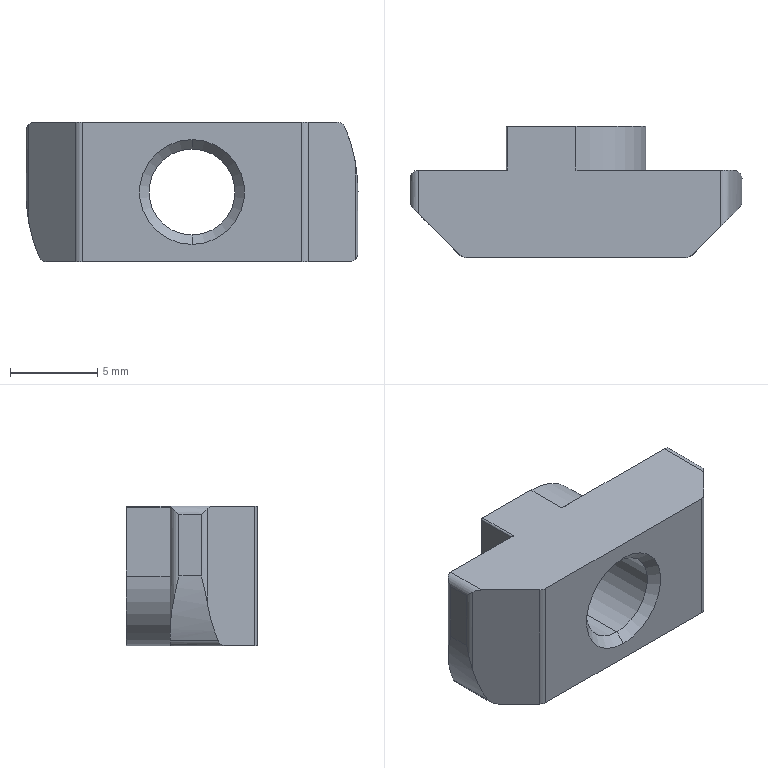Part | SolidWorks | features ICE 2, Extrusion 1, RevCut 1 | 1 solid | 34 faces | box 19 x 7.5 x 7.999 mm | volume 677.198 mm3 | cylinder 18 | plane 12 | cone 4 | commonest cylinder face diameters 1 x10 0.2 x2 4.917 x2 8 x2 19 x2
STEP:
#1=CARTESIAN_POINT('',(0.,0.5415,-2.458));
#2=VERTEX_POINT('',#1);
#3=CARTESIAN_POINT('',(0.,0.5415,2.458));
#4=VERTEX_POINT('',#3);
#5=CARTESIAN_POINT('',(0.,0.5415,0.));
#6=DIRECTION('',(0.,1.,0.));
#7=DIRECTION('',(0.,0.,1.));
#8=AXIS2_PLACEMENT_3D('',#5,#6,#7);
#9=CIRCLE('',#8,2.458);
#10=EDGE_CURVE('',#2,#4,#9,.T.);
#11=ORIENTED_EDGE('',*,*,#10,.T.);
#12=CARTESIAN_POINT('',(0.,0.,3.));
#13=VERTEX_POINT('',#12);
#14=CARTESIAN_POINT('',(0.,0.,3.));
#15=DIRECTION('',(0.,-0.7071,0.7071));
#16=VECTOR('',#15,1000.);
#17=LINE('',#14,#16);
#18=EDGE_CURVE('',#4,#13,#17,.T.);
#19=ORIENTED_EDGE('',*,*,#18,.T.);
#20=CARTESIAN_POINT('',(0.,0.,-3.));
#21=VERTEX_POINT('',#20);
#22=CARTESIAN_POINT('',(0.,0.,0.));
#23=DIRECTION('',(0.,1.,0.));
#24=DIRECTION('',(0.,0.,1.));
#25=AXIS2_PLACEMENT_3D('',#22,#23,#24);
#26=CIRCLE('',#25,3.);
#27=EDGE_CURVE('',#21,#13,#26,.T.);
#28=ORIENTED_EDGE('',*,*,#27,.F.);
#29=CARTESIAN_POINT('',(0.,0.,-3.));
#30=DIRECTION('',(0.,-0.7071,-0.7071));
#31=VECTOR('',#30,1000.);
#32=LINE('',#29,#31);
#33=EDGE_CURVE('',#2,#21,#32,.T.);
#34=ORIENTED_EDGE('',*,*,#33,.F.);
#35=EDGE_LOOP('',(#11,#19,#28,#34));
#36=FACE_OUTER_BOUND('',#35,.T.);
#37=CARTESIAN_POINT('',(0.,0.,0.));
#38=DIRECTION('',(0.,-1.,0.));
#39=DIRECTION('',(0.,0.,-1.));
#40=AXIS2_PLACEMENT_3D('',#37,#38,#39);
#41=CONICAL_SURFACE('',#40,3.,0.7854);
#42=ADVANCED_FACE('',(#36),#41,.F.);
#43=ORIENTED_EDGE('',*,*,#10,.F.);
#44=CARTESIAN_POINT('',(0.,6.958,-2.458));
#45=VERTEX_POINT('',#44);
#46=CARTESIAN_POINT('',(0.,0.,-2.458));
#47=DIRECTION('',(0.,1.,0.));
#48=VECTOR('',#47,1000.);
#49=LINE('',#46,#48);
#50=EDGE_CURVE('',#2,#45,#49,.T.);
#51=ORIENTED_EDGE('',*,*,#50,.T.);
#52=CARTESIAN_POINT('',(0.,6.958,2.458));
#53=VERTEX_POINT('',#52);
#54=CARTESIAN_POINT('',(0.,6.958,0.));
#55=DIRECTION('',(0.,1.,0.));
#56=DIRECTION('',(0.,0.,1.));
#57=AXIS2_PLACEMENT_3D('',#54,#55,#56);
#58=CIRCLE('',#57,2.458);
#59=EDGE_CURVE('',#45,#53,#58,.T.);
#60=ORIENTED_EDGE('',*,*,#59,.T.);
#61=CARTESIAN_POINT('',(0.,0.,2.458));
#62=DIRECTION('',(0.,1.,0.));
#63=VECTOR('',#62,1000.);
#64=LINE('',#61,#63);
#65=EDGE_CURVE('',#4,#53,#64,.T.);
#66=ORIENTED_EDGE('',*,*,#65,.F.);
#67=EDGE_LOOP('',(#43,#51,#60,#66));
#68=FACE_OUTER_BOUND('',#67,.T.);
#69=CARTESIAN_POINT('',(0.,0.,0.));
#70=DIRECTION('',(0.,1.,0.));
#71=DIRECTION('',(0.,0.,1.));
#72=AXIS2_PLACEMENT_3D('',#69,#70,#71);
#73=CYLINDRICAL_SURFACE('',#72,2.458);
#74=ADVANCED_FACE('',(#68),#73,.F.);
#75=ORIENTED_EDGE('',*,*,#59,.F.);
#76=CARTESIAN_POINT('',(0.,7.5,-3.));
#77=VERTEX_POINT('',#76);
#78=CARTESIAN_POINT('',(0.,6.958,-2.458));
#79=DIRECTION('',(0.,0.7071,-0.7071));
#80=VECTOR('',#79,1000.);
#81=LINE('',#78,#80);
#82=EDGE_CURVE('',#45,#77,#81,.T.);
#83=ORIENTED_EDGE('',*,*,#82,.T.);
#84=CARTESIAN_POINT('',(0.,7.5,3.));
#85=VERTEX_POINT('',#84);
#86=CARTESIAN_POINT('',(0.,7.5,0.));
#87=DIRECTION('',(0.,1.,0.));
#88=DIRECTION('',(0.,0.,1.));
#89=AXIS2_PLACEMENT_3D('',#86,#87,#88);
#90=CIRCLE('',#89,3.);
#91=EDGE_CURVE('',#77,#85,#90,.T.);
#92=ORIENTED_EDGE('',*,*,#91,.T.);
#93=CARTESIAN_POINT('',(0.,6.958,2.458));
#94=DIRECTION('',(0.,0.7071,0.7071));
#95=VECTOR('',#94,1000.);
#96=LINE('',#93,#95);
#97=EDGE_CURVE('',#53,#85,#96,.T.);
#98=ORIENTED_EDGE('',*,*,#97,.F.);
#99=EDGE_LOOP('',(#75,#83,#92,#98));
#100=FACE_OUTER_BOUND('',#99,.T.);
#101=CARTESIAN_POINT('',(0.,6.958,0.));
#102=DIRECTION('',(0.,1.,0.));
#103=DIRECTION('',(0.,0.,1.));
#104=AXIS2_PLACEMENT_3D('',#101,#102,#103);
#105=CONICAL_SURFACE('',#104,2.458,0.7854);
#106=ADVANCED_FACE('',(#100),#105,.F.);
#107=CARTESIAN_POINT('',(-6.646,0.1464,3.999));
#108=VERTEX_POINT('',#107);
#109=CARTESIAN_POINT('',(-9.,2.5,3.999));
#110=VERTEX_POINT('',#109);
#111=CARTESIAN_POINT('',(-9.354,2.854,3.999));
#112=DIRECTION('',(-0.7071,0.7071,0.));
#113=VECTOR('',#112,1000.);
#114=LINE('',#111,#113);
#115=EDGE_CURVE('',#108,#110,#114,.T.);
#116=ORIENTED_EDGE('',*,*,#115,.T.);
#117=CARTESIAN_POINT('',(-9.354,2.854,3.852));
#118=VERTEX_POINT('',#117);
#119=CARTESIAN_POINT('',(-9.,2.5,3.999));
#120=CARTESIAN_POINT('',(-9.134,2.634,3.999));
#121=CARTESIAN_POINT('',(-9.259,2.759,3.947));
#122=CARTESIAN_POINT('',(-9.354,2.854,3.852));
#123=(BOUNDED_CURVE()B_SPLINE_CURVE(3,(#119,#120,#121,#122),.UNSPECIFIED.,.F.,.F.)B_SPLINE_CURVE_WITH_KNOTS((4,4),(1.571,2.356),.UNSPECIFIED.)CURVE()GEOMETRIC_REPRESENTATION_ITEM()RATIONAL_B_SPLINE_CURVE((1.,0.9493,0.9493,1.))REPRESENTATION_ITEM(''));
#124=EDGE_CURVE('',#110,#118,#123,.T.);
#125=ORIENTED_EDGE('',*,*,#124,.T.);
#126=CARTESIAN_POINT('',(-9.354,2.854,-1.662));
#127=VERTEX_POINT('',#126);
#128=CARTESIAN_POINT('',(-9.354,2.854,4.));
#129=DIRECTION('',(0.,0.,-1.));
#130=VECTOR('',#129,1000.);
#131=LINE('',#128,#130);
#132=EDGE_CURVE('',#118,#127,#131,.T.);
#133=ORIENTED_EDGE('',*,*,#132,.T.);
#134=CARTESIAN_POINT('',(-8.752,2.252,-3.695));
#135=VERTEX_POINT('',#134);
#136=CARTESIAN_POINT('',(-9.354,2.854,-1.662));
#137=CARTESIAN_POINT('',(-9.229,2.729,-2.361));
#138=CARTESIAN_POINT('',(-9.028,2.528,-3.042));
#139=CARTESIAN_POINT('',(-8.752,2.252,-3.695));
#140=(BOUNDED_CURVE()B_SPLINE_CURVE(3,(#136,#137,#138,#139),.UNSPECIFIED.,.F.,.T.)B_SPLINE_CURVE_WITH_KNOTS((4,4),(3.317,3.541),.UNSPECIFIED.)CURVE()GEOMETRIC_REPRESENTATION_ITEM()RATIONAL_B_SPLINE_CURVE((1.,0.9958,0.9958,1.))REPRESENTATION_ITEM(''));
#141=EDGE_CURVE('',#127,#135,#140,.T.);
#142=ORIENTED_EDGE('',*,*,#141,.T.);
#143=CARTESIAN_POINT('',(-8.329,1.829,-4.));
#144=VERTEX_POINT('',#143);
#145=CARTESIAN_POINT('',(-8.752,2.252,-3.695));
#146=CARTESIAN_POINT('',(-8.677,2.177,-3.873));
#147=CARTESIAN_POINT('',(-8.521,2.021,-3.985));
#148=CARTESIAN_POINT('',(-8.329,1.829,-4.));
#149=(BOUNDED_CURVE()B_SPLINE_CURVE(3,(#145,#146,#147,#148),.UNSPECIFIED.,.F.,.F.)B_SPLINE_CURVE_WITH_KNOTS((4,4),(3.54,4.636),.UNSPECIFIED.)CURVE()GEOMETRIC_REPRESENTATION_ITEM()RATIONAL_B_SPLINE_CURVE((1.,0.9023,0.9023,1.))REPRESENTATION_ITEM(''));
#150=EDGE_CURVE('',#135,#144,#149,.T.);
#151=ORIENTED_EDGE('',*,*,#150,.T.);
#152=CARTESIAN_POINT('',(-6.646,0.1464,-4.));
#153=VERTEX_POINT('',#152);
#154=CARTESIAN_POINT('',(-9.354,2.854,-4.));
#155=DIRECTION('',(0.7071,-0.7071,0.));
#156=VECTOR('',#155,1000.);
#157=LINE('',#154,#156);
#158=EDGE_CURVE('',#144,#153,#157,.T.);
#159=ORIENTED_EDGE('',*,*,#158,.T.);
#160=CARTESIAN_POINT('',(-6.646,0.1464,4.));
#161=DIRECTION('',(0.,0.,-1.));
#162=VECTOR('',#161,1000.);
#163=LINE('',#160,#162);
#164=EDGE_CURVE('',#108,#153,#163,.T.);
#165=ORIENTED_EDGE('',*,*,#164,.F.);
#166=EDGE_LOOP('',(#116,#125,#133,#142,#151,#159,#165));
#167=FACE_OUTER_BOUND('',#166,.T.);
#168=CARTESIAN_POINT('',(-9.354,2.854,4.));
#169=DIRECTION('',(0.7071,0.7071,0.));
#170=DIRECTION('',(-0.7071,0.7071,0.));
#171=AXIS2_PLACEMENT_3D('',#168,#169,#170);
#172=PLANE('',#171);
#173=ADVANCED_FACE('',(#167),#172,.F.);
#174=CARTESIAN_POINT('',(8.753,2.252,3.693));
#175=VERTEX_POINT('',#174);
#176=CARTESIAN_POINT('',(8.292,1.791,3.999));
#177=VERTEX_POINT('',#176);
#178=CARTESIAN_POINT('',(8.753,2.252,3.693));
#179=CARTESIAN_POINT('',(8.672,2.171,3.884));
#180=CARTESIAN_POINT('',(8.5,1.999,3.999));
#181=CARTESIAN_POINT('',(8.292,1.791,3.999));
#182=(BOUNDED_CURVE()B_SPLINE_CURVE(3,(#178,#179,#180,#181),.UNSPECIFIED.,.F.,.F.)B_SPLINE_CURVE_WITH_KNOTS((4,4),(3.54,4.712),.UNSPECIFIED.)CURVE()GEOMETRIC_REPRESENTATION_ITEM()RATIONAL_B_SPLINE_CURVE((1.,0.8887,0.8887,1.))REPRESENTATION_ITEM(''));
#183=EDGE_CURVE('',#175,#177,#182,.T.);
#184=ORIENTED_EDGE('',*,*,#183,.T.);
#185=CARTESIAN_POINT('',(6.647,0.1464,3.999));
#186=VERTEX_POINT('',#185);
#187=CARTESIAN_POINT('',(6.647,0.1464,3.999));
#188=DIRECTION('',(-0.7071,-0.7071,0.));
#189=VECTOR('',#188,1000.);
#190=LINE('',#187,#189);
#191=EDGE_CURVE('',#177,#186,#190,.T.);
#192=ORIENTED_EDGE('',*,*,#191,.T.);
#193=CARTESIAN_POINT('',(6.647,0.1464,-4.));
#194=VERTEX_POINT('',#193);
#195=CARTESIAN_POINT('',(6.647,0.1464,4.));
#196=DIRECTION('',(0.,0.,-1.));
#197=VECTOR('',#196,1000.);
#198=LINE('',#195,#197);
#199=EDGE_CURVE('',#186,#194,#198,.T.);
#200=ORIENTED_EDGE('',*,*,#199,.T.);
#201=CARTESIAN_POINT('',(9.038,2.537,-4.));
#202=VERTEX_POINT('',#201);
#203=CARTESIAN_POINT('',(6.647,0.1464,-4.));
#204=DIRECTION('',(0.7071,0.7071,0.));
#205=VECTOR('',#204,1000.);
#206=LINE('',#203,#205);
#207=EDGE_CURVE('',#194,#202,#206,.T.);
#208=ORIENTED_EDGE('',*,*,#207,.T.);
#209=CARTESIAN_POINT('',(9.354,2.853,-3.855));
#210=VERTEX_POINT('',#209);
#211=CARTESIAN_POINT('',(9.038,2.537,-4.));
#212=CARTESIAN_POINT('',(9.158,2.657,-3.991));
#213=CARTESIAN_POINT('',(9.268,2.767,-3.94));
#214=CARTESIAN_POINT('',(9.354,2.853,-3.855));
#215=(BOUNDED_CURVE()B_SPLINE_CURVE(3,(#211,#212,#213,#214),.UNSPECIFIED.,.F.,.F.)B_SPLINE_CURVE_WITH_KNOTS((4,4),(1.647,2.356),.UNSPECIFIED.)CURVE()GEOMETRIC_REPRESENTATION_ITEM()RATIONAL_B_SPLINE_CURVE((1.,0.9585,0.9585,1.))REPRESENTATION_ITEM(''));
#216=EDGE_CURVE('',#202,#210,#215,.T.);
#217=ORIENTED_EDGE('',*,*,#216,.T.);
#218=CARTESIAN_POINT('',(9.354,2.853,1.662));
#219=VERTEX_POINT('',#218);
#220=CARTESIAN_POINT('',(9.354,2.853,4.));
#221=DIRECTION('',(0.,0.,-1.));
#222=VECTOR('',#221,1000.);
#223=LINE('',#220,#222);
#224=EDGE_CURVE('',#219,#210,#223,.T.);
#225=ORIENTED_EDGE('',*,*,#224,.F.);
#226=CARTESIAN_POINT('',(9.354,2.853,1.662));
#227=CARTESIAN_POINT('',(9.23,2.729,2.36));
#228=CARTESIAN_POINT('',(9.029,2.528,3.039));
#229=CARTESIAN_POINT('',(8.753,2.252,3.693));
#230=(BOUNDED_CURVE()B_SPLINE_CURVE(3,(#226,#227,#228,#229),.UNSPECIFIED.,.F.,.F.)B_SPLINE_CURVE_WITH_KNOTS((4,4),(3.317,3.541),.UNSPECIFIED.)CURVE()GEOMETRIC_REPRESENTATION_ITEM()RATIONAL_B_SPLINE_CURVE((1.,0.9958,0.9958,1.))REPRESENTATION_ITEM(''));
#231=EDGE_CURVE('',#219,#175,#230,.T.);
#232=ORIENTED_EDGE('',*,*,#231,.T.);
#233=EDGE_LOOP('',(#184,#192,#200,#208,#217,#225,#232));
#234=FACE_OUTER_BOUND('',#233,.T.);
#235=CARTESIAN_POINT('',(6.647,0.1464,4.));
#236=DIRECTION('',(-0.7071,0.7071,0.));
#237=DIRECTION('',(-0.7071,-0.7071,0.));
#238=AXIS2_PLACEMENT_3D('',#235,#236,#237);
#239=PLANE('',#238);
#240=ADVANCED_FACE('',(#234),#239,.F.);
#241=CARTESIAN_POINT('',(9.5,4.5,-3.501));
#242=VERTEX_POINT('',#241);
#243=CARTESIAN_POINT('',(9.5,3.206,-3.501));
#244=VERTEX_POINT('',#243);
#245=CARTESIAN_POINT('',(9.5,5.5,-3.501));
#246=DIRECTION('',(0.,-1.,0.));
#247=VECTOR('',#246,1000.);
#248=LINE('',#245,#247);
#249=EDGE_CURVE('',#242,#244,#248,.T.);
#250=ORIENTED_EDGE('',*,*,#249,.F.);
#251=CARTESIAN_POINT('',(9.5,4.5,0.));
#252=VERTEX_POINT('',#251);
#253=CARTESIAN_POINT('',(9.5,4.5,4.));
#254=DIRECTION('',(0.,0.,-1.));
#255=VECTOR('',#254,1000.);
#256=LINE('',#253,#255);
#257=EDGE_CURVE('',#252,#242,#256,.T.);
#258=ORIENTED_EDGE('',*,*,#257,.F.);
#259=CARTESIAN_POINT('',(9.5,3.206,0.));
#260=VERTEX_POINT('',#259);
#261=CARTESIAN_POINT('',(9.5,5.5,0.));
#262=DIRECTION('',(0.,1.,0.));
#263=VECTOR('',#262,1000.);
#264=LINE('',#261,#263);
#265=EDGE_CURVE('',#260,#252,#264,.T.);
#266=ORIENTED_EDGE('',*,*,#265,.F.);
#267=CARTESIAN_POINT('',(9.5,3.206,4.));
#268=DIRECTION('',(0.,0.,-1.));
#269=VECTOR('',#268,1000.);
#270=LINE('',#267,#269);
#271=EDGE_CURVE('',#260,#244,#270,.T.);
#272=ORIENTED_EDGE('',*,*,#271,.T.);
#273=EDGE_LOOP('',(#250,#258,#266,#272));
#274=FACE_OUTER_BOUND('',#273,.T.);
#275=CARTESIAN_POINT('',(9.5,3.206,4.));
#276=DIRECTION('',(-1.,0.,0.));
#277=DIRECTION('',(0.,0.,1.));
#278=AXIS2_PLACEMENT_3D('',#275,#276,#277);
#279=PLANE('',#278);
#280=ADVANCED_FACE('',(#274),#279,.F.);
#281=CARTESIAN_POINT('',(-9.,5.,3.999));
#282=VERTEX_POINT('',#281);
#283=CARTESIAN_POINT('',(-9.,5.,-3.042));
#284=VERTEX_POINT('',#283);
#285=CARTESIAN_POINT('',(-9.,5.,4.));
#286=DIRECTION('',(0.,0.,-1.));
#287=VECTOR('',#286,1000.);
#288=LINE('',#285,#287);
#289=EDGE_CURVE('',#282,#284,#288,.T.);
#290=ORIENTED_EDGE('',*,*,#289,.F.);
#291=CARTESIAN_POINT('',(-3.9,5.,3.999));
#292=VERTEX_POINT('',#291);
#293=CARTESIAN_POINT('',(-4.1,5.,3.999));
#294=DIRECTION('',(1.,0.,0.));
#295=VECTOR('',#294,1000.);
#296=LINE('',#293,#295);
#297=EDGE_CURVE('',#282,#292,#296,.T.);
#298=ORIENTED_EDGE('',*,*,#297,.T.);
#299=CARTESIAN_POINT('',(-4.,5.,3.899));
#300=VERTEX_POINT('',#299);
#301=CARTESIAN_POINT('',(-3.9,5.,3.899));
#302=DIRECTION('',(0.,1.,0.));
#303=DIRECTION('',(0.,0.,1.));
#304=AXIS2_PLACEMENT_3D('',#301,#302,#303);
#305=CIRCLE('',#304,0.1);
#306=EDGE_CURVE('',#300,#292,#305,.T.);
#307=ORIENTED_EDGE('',*,*,#306,.F.);
#308=CARTESIAN_POINT('',(-4.,5.,-0.001441));
#309=VERTEX_POINT('',#308);
#310=CARTESIAN_POINT('',(-4.,5.,-0.001441));
#311=DIRECTION('',(0.,0.,1.));
#312=VECTOR('',#311,1000.);
#313=LINE('',#310,#312);
#314=EDGE_CURVE('',#309,#300,#313,.T.);
#315=ORIENTED_EDGE('',*,*,#314,.F.);
#316=CARTESIAN_POINT('',(-0.1074,5.,-4.));
#317=VERTEX_POINT('',#316);
#318=CARTESIAN_POINT('',(-0.000000109,5.,-0.001441));
#319=DIRECTION('',(0.,1.,0.));
#320=DIRECTION('',(0.,0.,1.));
#321=AXIS2_PLACEMENT_3D('',#318,#319,#320);
#322=CIRCLE('',#321,4.);
#323=EDGE_CURVE('',#317,#309,#322,.T.);
#324=ORIENTED_EDGE('',*,*,#323,.F.);
#325=CARTESIAN_POINT('',(-8.329,5.,-4.));
#326=VERTEX_POINT('',#325);
#327=CARTESIAN_POINT('',(-4.1,5.,-4.));
#328=DIRECTION('',(-1.,0.,0.));
#329=VECTOR('',#328,1000.);
#330=LINE('',#327,#329);
#331=EDGE_CURVE('',#317,#326,#330,.T.);
#332=ORIENTED_EDGE('',*,*,#331,.T.);
#333=CARTESIAN_POINT('',(-8.752,5.,-3.695));
#334=VERTEX_POINT('',#333);
#335=CARTESIAN_POINT('',(-8.291,5.,-3.501));
#336=DIRECTION('',(0.,1.,0.));
#337=DIRECTION('',(0.,0.,-1.));
#338=AXIS2_PLACEMENT_3D('',#335,#336,#337);
#339=CIRCLE('',#338,0.5);
#340=EDGE_CURVE('',#326,#334,#339,.T.);
#341=ORIENTED_EDGE('',*,*,#340,.T.);
#342=CARTESIAN_POINT('',(-0.000000132,5.,-0.0005123));
#343=DIRECTION('',(0.,1.,0.));
#344=DIRECTION('',(0.,0.,-1.));
#345=AXIS2_PLACEMENT_3D('',#342,#343,#344);
#346=CIRCLE('',#345,9.5);
#347=EDGE_CURVE('',#334,#284,#346,.T.);
#348=ORIENTED_EDGE('',*,*,#347,.T.);
#349=EDGE_LOOP('',(#290,#298,#307,#315,#324,#332,#341,#348));
#350=FACE_OUTER_BOUND('',#349,.T.);
#351=CARTESIAN_POINT('',(-4.1,5.,4.));
#352=DIRECTION('',(0.,-1.,0.));
#353=DIRECTION('',(0.,0.,-1.));
#354=AXIS2_PLACEMENT_3D('',#351,#352,#353);
#355=PLANE('',#354);
#356=ADVANCED_FACE('',(#350),#355,.F.);
#357=CARTESIAN_POINT('',(-0.000000109,5.,3.999));
#358=VERTEX_POINT('',#357);
#359=CARTESIAN_POINT('',(4.,5.,-0.001441));
#360=VERTEX_POINT('',#359);
#361=CARTESIAN_POINT('',(-0.000000109,5.,-0.001441));
#362=DIRECTION('',(0.,1.,0.));
#363=DIRECTION('',(0.,0.,1.));
#364=AXIS2_PLACEMENT_3D('',#361,#362,#363);
#365=CIRCLE('',#364,4.);
#366=EDGE_CURVE('',#358,#360,#365,.T.);
#367=ORIENTED_EDGE('',*,*,#366,.F.);
#368=CARTESIAN_POINT('',(8.292,5.,3.999));
#369=VERTEX_POINT('',#368);
#370=CARTESIAN_POINT('',(-4.1,5.,3.999));
#371=DIRECTION('',(1.,0.,0.));
#372=VECTOR('',#371,1000.);
#373=LINE('',#370,#372);
#374=EDGE_CURVE('',#358,#369,#373,.T.);
#375=ORIENTED_EDGE('',*,*,#374,.T.);
#376=CARTESIAN_POINT('',(8.753,5.,3.693));
#377=VERTEX_POINT('',#376);
#378=CARTESIAN_POINT('',(8.292,5.,3.499));
#379=DIRECTION('',(0.,1.,0.));
#380=DIRECTION('',(0.,0.,-1.));
#381=AXIS2_PLACEMENT_3D('',#378,#379,#380);
#382=CIRCLE('',#381,0.5);
#383=EDGE_CURVE('',#369,#377,#382,.T.);
#384=ORIENTED_EDGE('',*,*,#383,.T.);
#385=CARTESIAN_POINT('',(9.,5.,3.041));
#386=VERTEX_POINT('',#385);
#387=CARTESIAN_POINT('',(0.,5.,0.));
#388=DIRECTION('',(0.,1.,0.));
#389=DIRECTION('',(0.,0.,-1.));
#390=AXIS2_PLACEMENT_3D('',#387,#388,#389);
#391=CIRCLE('',#390,9.5);
#392=EDGE_CURVE('',#377,#386,#391,.T.);
#393=ORIENTED_EDGE('',*,*,#392,.T.);
#394=CARTESIAN_POINT('',(9.,5.,-4.));
#395=VERTEX_POINT('',#394);
#396=CARTESIAN_POINT('',(9.,5.,4.));
#397=DIRECTION('',(0.,0.,-1.));
#398=VECTOR('',#397,1000.);
#399=LINE('',#396,#398);
#400=EDGE_CURVE('',#386,#395,#399,.T.);
#401=ORIENTED_EDGE('',*,*,#400,.T.);
#402=CARTESIAN_POINT('',(3.917,5.,-4.));
#403=VERTEX_POINT('',#402);
#404=CARTESIAN_POINT('',(9.,5.,-4.));
#405=DIRECTION('',(-1.,0.,0.));
#406=VECTOR('',#405,1000.);
#407=LINE('',#404,#406);
#408=EDGE_CURVE('',#395,#403,#407,.T.);
#409=ORIENTED_EDGE('',*,*,#408,.T.);
#410=CARTESIAN_POINT('',(4.,5.,-3.901));
#411=VERTEX_POINT('',#410);
#412=CARTESIAN_POINT('',(3.9,5.,-3.901));
#413=DIRECTION('',(0.,1.,0.));
#414=DIRECTION('',(0.,0.,1.));
#415=AXIS2_PLACEMENT_3D('',#412,#413,#414);
#416=CIRCLE('',#415,0.1);
#417=EDGE_CURVE('',#411,#403,#416,.T.);
#418=ORIENTED_EDGE('',*,*,#417,.F.);
#419=CARTESIAN_POINT('',(4.,5.,-0.001441));
#420=DIRECTION('',(0.,0.,-1.));
#421=VECTOR('',#420,1000.);
#422=LINE('',#419,#421);
#423=EDGE_CURVE('',#360,#411,#422,.T.);
#424=ORIENTED_EDGE('',*,*,#423,.F.);
#425=EDGE_LOOP('',(#367,#375,#384,#393,#401,#409,#418,#424));
#426=FACE_OUTER_BOUND('',#425,.T.);
#427=CARTESIAN_POINT('',(-4.1,5.,4.));
#428=DIRECTION('',(0.,-1.,0.));
#429=DIRECTION('',(0.,0.,-1.));
#430=AXIS2_PLACEMENT_3D('',#427,#428,#429);
#431=PLANE('',#430);
#432=ADVANCED_FACE('',(#426),#431,.F.);
#433=CARTESIAN_POINT('',(-9.5,3.207,3.499));
#434=VERTEX_POINT('',#433);
#435=CARTESIAN_POINT('',(-9.5,3.207,-0.0005123));
#436=VERTEX_POINT('',#435);
#437=CARTESIAN_POINT('',(-9.5,3.207,4.));
#438=DIRECTION('',(0.,0.,-1.));
#439=VECTOR('',#438,1000.);
#440=LINE('',#437,#439);
#441=EDGE_CURVE('',#434,#436,#440,.T.);
#442=ORIENTED_EDGE('',*,*,#441,.F.);
#443=CARTESIAN_POINT('',(-9.5,4.5,3.499));
#444=VERTEX_POINT('',#443);
#445=CARTESIAN_POINT('',(-9.5,5.5,3.499));
#446=DIRECTION('',(0.,1.,0.));
#447=VECTOR('',#446,1000.);
#448=LINE('',#445,#447);
#449=EDGE_CURVE('',#434,#444,#448,.T.);
#450=ORIENTED_EDGE('',*,*,#449,.T.);
#451=CARTESIAN_POINT('',(-9.5,4.5,-0.0005123));
#452=VERTEX_POINT('',#451);
#453=CARTESIAN_POINT('',(-9.5,4.5,4.));
#454=DIRECTION('',(0.,0.,-1.));
#455=VECTOR('',#454,1000.);
#456=LINE('',#453,#455);
#457=EDGE_CURVE('',#444,#452,#456,.T.);
#458=ORIENTED_EDGE('',*,*,#457,.T.);
#459=CARTESIAN_POINT('',(-9.5,5.5,-0.0005123));
#460=DIRECTION('',(0.,1.,0.));
#461=VECTOR('',#460,1000.);
#462=LINE('',#459,#461);
#463=EDGE_CURVE('',#436,#452,#462,.T.);
#464=ORIENTED_EDGE('',*,*,#463,.F.);
#465=EDGE_LOOP('',(#442,#450,#458,#464));
#466=FACE_OUTER_BOUND('',#465,.T.);
#467=CARTESIAN_POINT('',(-9.5,4.5,4.));
#468=DIRECTION('',(1.,0.,0.));
#469=DIRECTION('',(0.,0.,-1.));
#470=AXIS2_PLACEMENT_3D('',#467,#468,#469);
#471=PLANE('',#470);
#472=ADVANCED_FACE('',(#466),#471,.F.);
#473=CARTESIAN_POINT('',(4.,7.5,-0.001441));
#474=VERTEX_POINT('',#473);
#475=CARTESIAN_POINT('',(4.,11.,-0.001441));
#476=DIRECTION('',(0.,-1.,0.));
#477=VECTOR('',#476,1000.);
#478=LINE('',#475,#477);
#479=EDGE_CURVE('',#474,#360,#478,.T.);
#480=ORIENTED_EDGE('',*,*,#479,.T.);
#481=ORIENTED_EDGE('',*,*,#423,.T.);
#482=CARTESIAN_POINT('',(4.,7.5,-3.901));
#483=VERTEX_POINT('',#482);
#484=CARTESIAN_POINT('',(4.,11.,-3.901));
#485=DIRECTION('',(0.,-1.,0.));
#486=VECTOR('',#485,1000.);
#487=LINE('',#484,#486);
#488=EDGE_CURVE('',#483,#411,#487,.T.);
#489=ORIENTED_EDGE('',*,*,#488,.F.);
#490=CARTESIAN_POINT('',(4.,7.5,4.));
#491=DIRECTION('',(0.,0.,-1.));
#492=VECTOR('',#491,1000.);
#493=LINE('',#490,#492);
#494=EDGE_CURVE('',#474,#483,#493,.T.);
#495=ORIENTED_EDGE('',*,*,#494,.F.);
#496=EDGE_LOOP('',(#480,#481,#489,#495));
#497=FACE_OUTER_BOUND('',#496,.T.);
#498=CARTESIAN_POINT('',(4.,5.1,4.));
#499=DIRECTION('',(-1.,0.,0.));
#500=DIRECTION('',(0.,0.,1.));
#501=AXIS2_PLACEMENT_3D('',#498,#499,#500);
#502=PLANE('',#501);
#503=ADVANCED_FACE('',(#497),#502,.F.);
#504=CARTESIAN_POINT('',(0.,7.5,0.));
#505=DIRECTION('',(0.,1.,0.));
#506=DIRECTION('',(0.,0.,1.));
#507=AXIS2_PLACEMENT_3D('',#504,#505,#506);
#508=CIRCLE('',#507,3.);
#509=EDGE_CURVE('',#85,#77,#508,.T.);
#510=ORIENTED_EDGE('',*,*,#509,.F.);
#511=ORIENTED_EDGE('',*,*,#91,.F.);
#512=EDGE_LOOP('',(#510,#511));
#513=FACE_BOUND('',#512,.T.);
#514=CARTESIAN_POINT('',(3.917,7.5,-4.));
#515=VERTEX_POINT('',#514);
#516=CARTESIAN_POINT('',(-0.1074,7.5,-4.));
#517=VERTEX_POINT('',#516);
#518=CARTESIAN_POINT('',(4.,7.5,-4.));
#519=DIRECTION('',(-1.,0.,0.));
#520=VECTOR('',#519,1000.);
#521=LINE('',#518,#520);
#522=EDGE_CURVE('',#515,#517,#521,.T.);
#523=ORIENTED_EDGE('',*,*,#522,.T.);
#524=CARTESIAN_POINT('',(-4.,7.5,-0.001441));
#525=VERTEX_POINT('',#524);
#526=CARTESIAN_POINT('',(-0.000000109,7.5,-0.001441));
#527=DIRECTION('',(0.,1.,0.));
#528=DIRECTION('',(0.,0.,-1.));
#529=AXIS2_PLACEMENT_3D('',#526,#527,#528);
#530=CIRCLE('',#529,4.);
#531=EDGE_CURVE('',#517,#525,#530,.T.);
#532=ORIENTED_EDGE('',*,*,#531,.T.);
#533=CARTESIAN_POINT('',(-4.,7.5,3.899));
#534=VERTEX_POINT('',#533);
#535=CARTESIAN_POINT('',(-4.,7.5,4.));
#536=DIRECTION('',(0.,0.,-1.));
#537=VECTOR('',#536,1000.);
#538=LINE('',#535,#537);
#539=EDGE_CURVE('',#534,#525,#538,.T.);
#540=ORIENTED_EDGE('',*,*,#539,.F.);
#541=CARTESIAN_POINT('',(-3.9,7.5,3.999));
#542=VERTEX_POINT('',#541);
#543=CARTESIAN_POINT('',(-3.9,7.5,3.899));
#544=DIRECTION('',(0.,1.,0.));
#545=DIRECTION('',(0.,0.,-1.));
#546=AXIS2_PLACEMENT_3D('',#543,#544,#545);
#547=CIRCLE('',#546,0.1);
#548=EDGE_CURVE('',#534,#542,#547,.T.);
#549=ORIENTED_EDGE('',*,*,#548,.T.);
#550=CARTESIAN_POINT('',(-0.000000109,7.5,3.999));
#551=VERTEX_POINT('',#550);
#552=CARTESIAN_POINT('',(4.,7.5,3.999));
#553=DIRECTION('',(1.,0.,0.));
#554=VECTOR('',#553,1000.);
#555=LINE('',#552,#554);
#556=EDGE_CURVE('',#542,#551,#555,.T.);
#557=ORIENTED_EDGE('',*,*,#556,.T.);
#558=CARTESIAN_POINT('',(-0.000000109,7.5,-0.001441));
#559=DIRECTION('',(0.,1.,0.));
#560=DIRECTION('',(0.,0.,-1.));
#561=AXIS2_PLACEMENT_3D('',#558,#559,#560);
#562=CIRCLE('',#561,4.);
#563=EDGE_CURVE('',#551,#474,#562,.T.);
#564=ORIENTED_EDGE('',*,*,#563,.T.);
#565=ORIENTED_EDGE('',*,*,#494,.T.);
#566=CARTESIAN_POINT('',(3.9,7.5,-3.901));
#567=DIRECTION('',(0.,1.,0.));
#568=DIRECTION('',(0.,0.,-1.));
#569=AXIS2_PLACEMENT_3D('',#566,#567,#568);
#570=CIRCLE('',#569,0.1);
#571=EDGE_CURVE('',#483,#515,#570,.T.);
#572=ORIENTED_EDGE('',*,*,#571,.T.);
#573=EDGE_LOOP('',(#523,#532,#540,#549,#557,#564,#565,#572));
#574=FACE_OUTER_BOUND('',#573,.T.);
#575=CARTESIAN_POINT('',(4.,7.5,4.));
#576=DIRECTION('',(0.,-1.,0.));
#577=DIRECTION('',(0.,0.,-1.));
#578=AXIS2_PLACEMENT_3D('',#575,#576,#577);
#579=PLANE('',#578);
#580=ADVANCED_FACE('',(#513,#574),#579,.F.);
#581=CARTESIAN_POINT('',(-4.,11.,-0.001441));
#582=DIRECTION('',(0.,-1.,0.));
#583=VECTOR('',#582,1000.);
#584=LINE('',#581,#583);
#585=EDGE_CURVE('',#525,#309,#584,.T.);
#586=ORIENTED_EDGE('',*,*,#585,.T.);
#587=ORIENTED_EDGE('',*,*,#314,.T.);
#588=CARTESIAN_POINT('',(-4.,11.,3.899));
#589=DIRECTION('',(0.,-1.,0.));
#590=VECTOR('',#589,1000.);
#591=LINE('',#588,#590);
#592=EDGE_CURVE('',#534,#300,#591,.T.);
#593=ORIENTED_EDGE('',*,*,#592,.F.);
#594=ORIENTED_EDGE('',*,*,#539,.T.);
#595=EDGE_LOOP('',(#586,#587,#593,#594));
#596=FACE_OUTER_BOUND('',#595,.T.);
#597=CARTESIAN_POINT('',(-4.,7.5,4.));
#598=DIRECTION('',(1.,0.,0.));
#599=DIRECTION('',(0.,0.,-1.));
#600=AXIS2_PLACEMENT_3D('',#597,#598,#599);
#601=PLANE('',#600);
#602=ADVANCED_FACE('',(#596),#601,.F.);
#603=CARTESIAN_POINT('',(9.038,4.999,-4.));
#604=VERTEX_POINT('',#603);
#605=CARTESIAN_POINT('',(9.,4.5,-4.));
#606=DIRECTION('',(0.,0.,1.));
#607=DIRECTION('',(1.,0.,0.));
#608=AXIS2_PLACEMENT_3D('',#605,#606,#607);
#609=CIRCLE('',#608,0.5);
#610=EDGE_CURVE('',#604,#395,#609,.T.);
#611=ORIENTED_EDGE('',*,*,#610,.F.);
#612=CARTESIAN_POINT('',(9.038,5.5,-4.));
#613=DIRECTION('',(0.,-1.,0.));
#614=VECTOR('',#613,1000.);
#615=LINE('',#612,#614);
#616=EDGE_CURVE('',#604,#202,#615,.T.);
#617=ORIENTED_EDGE('',*,*,#616,.T.);
#618=ORIENTED_EDGE('',*,*,#207,.F.);
#619=CARTESIAN_POINT('',(6.294,0.,-4.));
#620=VERTEX_POINT('',#619);
#621=CARTESIAN_POINT('',(6.294,0.5,-4.));
#622=DIRECTION('',(0.,0.,1.));
#623=DIRECTION('',(1.,0.,0.));
#624=AXIS2_PLACEMENT_3D('',#621,#622,#623);
#625=CIRCLE('',#624,0.5);
#626=EDGE_CURVE('',#620,#194,#625,.T.);
#627=ORIENTED_EDGE('',*,*,#626,.F.);
#628=CARTESIAN_POINT('',(-6.293,0.,-4.));
#629=VERTEX_POINT('',#628);
#630=CARTESIAN_POINT('',(-6.293,0.,-4.));
#631=DIRECTION('',(1.,0.,0.));
#632=VECTOR('',#631,1000.);
#633=LINE('',#630,#632);
#634=EDGE_CURVE('',#629,#620,#633,.T.);
#635=ORIENTED_EDGE('',*,*,#634,.F.);
#636=CARTESIAN_POINT('',(-6.293,0.5,-4.));
#637=DIRECTION('',(0.,0.,1.));
#638=DIRECTION('',(1.,0.,0.));
#639=AXIS2_PLACEMENT_3D('',#636,#637,#638);
#640=CIRCLE('',#639,0.5);
#641=EDGE_CURVE('',#153,#629,#640,.T.);
#642=ORIENTED_EDGE('',*,*,#641,.F.);
#643=ORIENTED_EDGE('',*,*,#158,.F.);
#644=CARTESIAN_POINT('',(-8.329,5.5,-4.));
#645=DIRECTION('',(0.,1.,0.));
#646=VECTOR('',#645,1000.);
#647=LINE('',#644,#646);
#648=EDGE_CURVE('',#144,#326,#647,.T.);
#649=ORIENTED_EDGE('',*,*,#648,.T.);
#650=ORIENTED_EDGE('',*,*,#331,.F.);
#651=CARTESIAN_POINT('',(-0.1074,11.,-4.));
#652=DIRECTION('',(0.,1.,0.));
#653=VECTOR('',#652,1000.);
#654=LINE('',#651,#653);
#655=EDGE_CURVE('',#317,#517,#654,.T.);
#656=ORIENTED_EDGE('',*,*,#655,.T.);
#657=ORIENTED_EDGE('',*,*,#522,.F.);
#658=CARTESIAN_POINT('',(3.917,11.,-4.));
#659=DIRECTION('',(0.,-1.,0.));
#660=VECTOR('',#659,1000.);
#661=LINE('',#658,#660);
#662=EDGE_CURVE('',#515,#403,#661,.T.);
#663=ORIENTED_EDGE('',*,*,#662,.T.);
#664=ORIENTED_EDGE('',*,*,#408,.F.);
#665=EDGE_LOOP('',(#611,#617,#618,#627,#635,#642,#643,#649,#650,#656,#657,#663,#664));
#666=FACE_OUTER_BOUND('',#665,.T.);
#667=CARTESIAN_POINT('',(-9.,3.207,-4.));
#668=DIRECTION('',(0.,0.,1.));
#669=DIRECTION('',(1.,0.,0.));
#670=AXIS2_PLACEMENT_3D('',#667,#668,#669);
#671=PLANE('',#670);
#672=ADVANCED_FACE('',(#666),#671,.F.);
#673=ORIENTED_EDGE('',*,*,#132,.F.);
#674=CARTESIAN_POINT('',(-9.354,2.854,3.852));
#675=CARTESIAN_POINT('',(-9.449,2.949,3.757));
#676=CARTESIAN_POINT('',(-9.5,3.073,3.633));
#677=CARTESIAN_POINT('',(-9.5,3.207,3.499));
#678=(BOUNDED_CURVE()B_SPLINE_CURVE(3,(#674,#675,#676,#677),.UNSPECIFIED.,.F.,.F.)B_SPLINE_CURVE_WITH_KNOTS((4,4),(3.927,4.712),.UNSPECIFIED.)CURVE()GEOMETRIC_REPRESENTATION_ITEM()RATIONAL_B_SPLINE_CURVE((1.,0.9493,0.9493,1.))REPRESENTATION_ITEM(''));
#679=EDGE_CURVE('',#118,#434,#678,.T.);
#680=ORIENTED_EDGE('',*,*,#679,.T.);
#681=ORIENTED_EDGE('',*,*,#441,.T.);
#682=CARTESIAN_POINT('',(-9.5,3.207,-0.0005123));
#683=CARTESIAN_POINT('',(-9.5,3.08,-0.5554));
#684=CARTESIAN_POINT('',(-9.452,2.952,-1.11));
#685=CARTESIAN_POINT('',(-9.354,2.854,-1.662));
#686=B_SPLINE_CURVE_WITH_KNOTS('',3,(#682,#683,#684,#685),.UNSPECIFIED.,.F.,.F.,(4,4),(-0.00001949,0.001688),.UNSPECIFIED.);
#687=EDGE_CURVE('',#436,#127,#686,.T.);
#688=ORIENTED_EDGE('',*,*,#687,.T.);
#689=EDGE_LOOP('',(#673,#680,#681,#688));
#690=FACE_OUTER_BOUND('',#689,.T.);
#691=CARTESIAN_POINT('',(-9.,3.207,4.));
#692=DIRECTION('',(0.,0.,-1.));
#693=DIRECTION('',(-1.,0.,0.));
#694=AXIS2_PLACEMENT_3D('',#691,#692,#693);
#695=CYLINDRICAL_SURFACE('',#694,0.5);
#696=ADVANCED_FACE('',(#690),#695,.T.);
#697=CARTESIAN_POINT('',(-6.293,0.,3.999));
#698=VERTEX_POINT('',#697);
#699=CARTESIAN_POINT('',(-6.293,0.,4.));
#700=DIRECTION('',(0.,0.,-1.));
#701=VECTOR('',#700,1000.);
#702=LINE('',#699,#701);
#703=EDGE_CURVE('',#698,#629,#702,.T.);
#704=ORIENTED_EDGE('',*,*,#703,.F.);
#705=CARTESIAN_POINT('',(-6.293,0.5,3.999));
#706=DIRECTION('',(0.,0.,-1.));
#707=DIRECTION('',(-1.,0.,0.));
#708=AXIS2_PLACEMENT_3D('',#705,#706,#707);
#709=CIRCLE('',#708,0.5);
#710=EDGE_CURVE('',#698,#108,#709,.T.);
#711=ORIENTED_EDGE('',*,*,#710,.T.);
#712=ORIENTED_EDGE('',*,*,#164,.T.);
#713=ORIENTED_EDGE('',*,*,#641,.T.);
#714=EDGE_LOOP('',(#704,#711,#712,#713));
#715=FACE_OUTER_BOUND('',#714,.T.);
#716=CARTESIAN_POINT('',(-6.293,0.5,4.));
#717=DIRECTION('',(0.,0.,-1.));
#718=DIRECTION('',(-1.,0.,0.));
#719=AXIS2_PLACEMENT_3D('',#716,#717,#718);
#720=CYLINDRICAL_SURFACE('',#719,0.5);
#721=ADVANCED_FACE('',(#715),#720,.T.);
#722=ORIENTED_EDGE('',*,*,#27,.T.);
#723=CARTESIAN_POINT('',(0.,0.,0.));
#724=DIRECTION('',(0.,1.,0.));
#725=DIRECTION('',(0.,0.,1.));
#726=AXIS2_PLACEMENT_3D('',#723,#724,#725);
#727=CIRCLE('',#726,3.);
#728=EDGE_CURVE('',#13,#21,#727,.T.);
#729=ORIENTED_EDGE('',*,*,#728,.T.);
#730=EDGE_LOOP('',(#722,#729));
#731=FACE_BOUND('',#730,.T.);
#732=CARTESIAN_POINT('',(6.294,0.,3.999));
#733=VERTEX_POINT('',#732);
#734=CARTESIAN_POINT('',(6.294,0.,4.));
#735=DIRECTION('',(0.,0.,-1.));
#736=VECTOR('',#735,1000.);
#737=LINE('',#734,#736);
#738=EDGE_CURVE('',#733,#620,#737,.T.);
#739=ORIENTED_EDGE('',*,*,#738,.F.);
#740=CARTESIAN_POINT('',(-9.,0.,3.999));
#741=DIRECTION('',(1.,0.,0.));
#742=VECTOR('',#741,1000.);
#743=LINE('',#740,#742);
#744=EDGE_CURVE('',#698,#733,#743,.T.);
#745=ORIENTED_EDGE('',*,*,#744,.F.);
#746=ORIENTED_EDGE('',*,*,#703,.T.);
#747=ORIENTED_EDGE('',*,*,#634,.T.);
#748=EDGE_LOOP('',(#739,#745,#746,#747));
#749=FACE_OUTER_BOUND('',#748,.T.);
#750=CARTESIAN_POINT('',(-6.293,0.,4.));
#751=DIRECTION('',(0.,1.,0.));
#752=DIRECTION('',(0.,0.,1.));
#753=AXIS2_PLACEMENT_3D('',#750,#751,#752);
#754=PLANE('',#753);
#755=ADVANCED_FACE('',(#731,#749),#754,.F.);
#756=ORIENTED_EDGE('',*,*,#199,.F.);
#757=CARTESIAN_POINT('',(6.294,0.5,3.999));
#758=DIRECTION('',(0.,0.,-1.));
#759=DIRECTION('',(-1.,0.,0.));
#760=AXIS2_PLACEMENT_3D('',#757,#758,#759);
#761=CIRCLE('',#760,0.5);
#762=EDGE_CURVE('',#186,#733,#761,.T.);
#763=ORIENTED_EDGE('',*,*,#762,.T.);
#764=ORIENTED_EDGE('',*,*,#738,.T.);
#765=ORIENTED_EDGE('',*,*,#626,.T.);
#766=EDGE_LOOP('',(#756,#763,#764,#765));
#767=FACE_OUTER_BOUND('',#766,.T.);
#768=CARTESIAN_POINT('',(6.294,0.5,4.));
#769=DIRECTION('',(0.,0.,-1.));
#770=DIRECTION('',(-1.,0.,0.));
#771=AXIS2_PLACEMENT_3D('',#768,#769,#770);
#772=CYLINDRICAL_SURFACE('',#771,0.5);
#773=ADVANCED_FACE('',(#767),#772,.T.);
#774=CARTESIAN_POINT('',(9.354,2.853,-3.855));
#775=CARTESIAN_POINT('',(9.449,2.948,-3.76));
#776=CARTESIAN_POINT('',(9.5,3.072,-3.636));
#777=CARTESIAN_POINT('',(9.5,3.206,-3.501));
#778=(BOUNDED_CURVE()B_SPLINE_CURVE(3,(#774,#775,#776,#777),.UNSPECIFIED.,.F.,.F.)B_SPLINE_CURVE_WITH_KNOTS((4,4),(0.7854,1.571),.UNSPECIFIED.)CURVE()GEOMETRIC_REPRESENTATION_ITEM()RATIONAL_B_SPLINE_CURVE((1.,0.9493,0.9493,1.))REPRESENTATION_ITEM(''));
#779=EDGE_CURVE('',#210,#244,#778,.T.);
#780=ORIENTED_EDGE('',*,*,#779,.T.);
#781=ORIENTED_EDGE('',*,*,#271,.F.);
#782=CARTESIAN_POINT('',(9.5,3.206,0.));
#783=CARTESIAN_POINT('',(9.5,3.079,0.5548));
#784=CARTESIAN_POINT('',(9.452,2.951,1.109));
#785=CARTESIAN_POINT('',(9.354,2.853,1.662));
#786=B_SPLINE_CURVE_WITH_KNOTS('',3,(#782,#783,#784,#785),.UNSPECIFIED.,.F.,.F.,(4,4),(-0.00001949,0.001688),.UNSPECIFIED.);
#787=EDGE_CURVE('',#260,#219,#786,.T.);
#788=ORIENTED_EDGE('',*,*,#787,.T.);
#789=ORIENTED_EDGE('',*,*,#224,.T.);
#790=EDGE_LOOP('',(#780,#781,#788,#789));
#791=FACE_OUTER_BOUND('',#790,.T.);
#792=CARTESIAN_POINT('',(9.,3.206,4.));
#793=DIRECTION('',(0.,0.,-1.));
#794=DIRECTION('',(-1.,0.,0.));
#795=AXIS2_PLACEMENT_3D('',#792,#793,#794);
#796=CYLINDRICAL_SURFACE('',#795,0.5);
#797=ADVANCED_FACE('',(#791),#796,.T.);
#798=ORIENTED_EDGE('',*,*,#257,.T.);
#799=CARTESIAN_POINT('',(9.5,4.5,-3.501));
#800=CARTESIAN_POINT('',(9.5,4.776,-3.777));
#801=CARTESIAN_POINT('',(9.313,4.978,-3.979));
#802=CARTESIAN_POINT('',(9.038,4.999,-4.));
#803=(BOUNDED_CURVE()B_SPLINE_CURVE(3,(#799,#800,#801,#802),.UNSPECIFIED.,.F.,.F.)B_SPLINE_CURVE_WITH_KNOTS((4,4),(4.712,6.207),.UNSPECIFIED.)CURVE()GEOMETRIC_REPRESENTATION_ITEM()RATIONAL_B_SPLINE_CURVE((1.,0.8223,0.8223,1.))REPRESENTATION_ITEM(''));
#804=EDGE_CURVE('',#242,#604,#803,.T.);
#805=ORIENTED_EDGE('',*,*,#804,.T.);
#806=ORIENTED_EDGE('',*,*,#610,.T.);
#807=ORIENTED_EDGE('',*,*,#400,.F.);
#808=CARTESIAN_POINT('',(9.,5.,3.041));
#809=CARTESIAN_POINT('',(9.084,5.,2.792));
#810=CARTESIAN_POINT('',(9.158,4.98,2.541));
#811=CARTESIAN_POINT('',(9.283,4.918,2.035));
#812=CARTESIAN_POINT('',(9.335,4.876,1.781));
#813=CARTESIAN_POINT('',(9.459,4.734,1.019));
#814=CARTESIAN_POINT('',(9.5,4.617,0.511));
#815=CARTESIAN_POINT('',(9.5,4.5,0.));
#816=B_SPLINE_CURVE_WITH_KNOTS('',3,(#808,#809,#810,#811,#812,#813,#814,#815),.UNSPECIFIED.,.F.,.F.,(4,2,2,4),(0.,0.0007864,0.001573,0.003146),.UNSPECIFIED.);
#817=EDGE_CURVE('',#386,#252,#816,.T.);
#818=ORIENTED_EDGE('',*,*,#817,.T.);
#819=EDGE_LOOP('',(#798,#805,#806,#807,#818));
#820=FACE_OUTER_BOUND('',#819,.T.);
#821=CARTESIAN_POINT('',(9.,4.5,4.));
#822=DIRECTION('',(0.,0.,-1.));
#823=DIRECTION('',(-1.,0.,0.));
#824=AXIS2_PLACEMENT_3D('',#821,#822,#823);
#825=CYLINDRICAL_SURFACE('',#824,0.5);
#826=ADVANCED_FACE('',(#820),#825,.T.);
#827=ORIENTED_EDGE('',*,*,#457,.F.);
#828=CARTESIAN_POINT('',(-9.5,4.5,3.499));
#829=CARTESIAN_POINT('',(-9.5,4.793,3.791));
#830=CARTESIAN_POINT('',(-9.293,5.,3.999));
#831=CARTESIAN_POINT('',(-9.,5.,3.999));
#832=(BOUNDED_CURVE()B_SPLINE_CURVE(3,(#828,#829,#830,#831),.UNSPECIFIED.,.F.,.F.)B_SPLINE_CURVE_WITH_KNOTS((4,4),(1.571,3.142),.UNSPECIFIED.)CURVE()GEOMETRIC_REPRESENTATION_ITEM()RATIONAL_B_SPLINE_CURVE((1.,0.8047,0.8047,1.))REPRESENTATION_ITEM(''));
#833=EDGE_CURVE('',#444,#282,#832,.T.);
#834=ORIENTED_EDGE('',*,*,#833,.T.);
#835=ORIENTED_EDGE('',*,*,#289,.T.);
#836=CARTESIAN_POINT('',(-9.,5.,-3.042));
#837=CARTESIAN_POINT('',(-9.084,5.,-2.792));
#838=CARTESIAN_POINT('',(-9.158,4.98,-2.542));
#839=CARTESIAN_POINT('',(-9.283,4.918,-2.036));
#840=CARTESIAN_POINT('',(-9.335,4.876,-1.781));
#841=CARTESIAN_POINT('',(-9.459,4.734,-1.02));
#842=CARTESIAN_POINT('',(-9.5,4.617,-0.5116));
#843=CARTESIAN_POINT('',(-9.5,4.5,-0.0005123));
#844=B_SPLINE_CURVE_WITH_KNOTS('',3,(#836,#837,#838,#839,#840,#841,#842,#843),.UNSPECIFIED.,.F.,.F.,(4,2,2,4),(0.,0.0007864,0.001573,0.003146),.UNSPECIFIED.);
#845=EDGE_CURVE('',#284,#452,#844,.T.);
#846=ORIENTED_EDGE('',*,*,#845,.T.);
#847=EDGE_LOOP('',(#827,#834,#835,#846));
#848=FACE_OUTER_BOUND('',#847,.T.);
#849=CARTESIAN_POINT('',(-9.,4.5,4.));
#850=DIRECTION('',(0.,0.,-1.));
#851=DIRECTION('',(-1.,0.,0.));
#852=AXIS2_PLACEMENT_3D('',#849,#850,#851);
#853=CYLINDRICAL_SURFACE('',#852,0.5);
#854=ADVANCED_FACE('',(#848),#853,.T.);
#855=ORIENTED_EDGE('',*,*,#82,.F.);
#856=CARTESIAN_POINT('',(0.,6.958,0.));
#857=DIRECTION('',(0.,1.,0.));
#858=DIRECTION('',(0.,0.,1.));
#859=AXIS2_PLACEMENT_3D('',#856,#857,#858);
#860=CIRCLE('',#859,2.458);
#861=EDGE_CURVE('',#53,#45,#860,.T.);
#862=ORIENTED_EDGE('',*,*,#861,.F.);
#863=ORIENTED_EDGE('',*,*,#97,.T.);
#864=ORIENTED_EDGE('',*,*,#509,.T.);
#865=EDGE_LOOP('',(#855,#862,#863,#864));
#866=FACE_OUTER_BOUND('',#865,.T.);
#867=CARTESIAN_POINT('',(0.,6.958,0.));
#868=DIRECTION('',(0.,1.,0.));
#869=DIRECTION('',(0.,0.,1.));
#870=AXIS2_PLACEMENT_3D('',#867,#868,#869);
#871=CONICAL_SURFACE('',#870,2.458,0.7854);
#872=ADVANCED_FACE('',(#866),#871,.F.);
#873=ORIENTED_EDGE('',*,*,#50,.F.);
#874=CARTESIAN_POINT('',(0.,0.5415,0.));
#875=DIRECTION('',(0.,1.,0.));
#876=DIRECTION('',(0.,0.,1.));
#877=AXIS2_PLACEMENT_3D('',#874,#875,#876);
#878=CIRCLE('',#877,2.458);
#879=EDGE_CURVE('',#4,#2,#878,.T.);
#880=ORIENTED_EDGE('',*,*,#879,.F.);
#881=ORIENTED_EDGE('',*,*,#65,.T.);
#882=ORIENTED_EDGE('',*,*,#861,.T.);
#883=EDGE_LOOP('',(#873,#880,#881,#882));
#884=FACE_OUTER_BOUND('',#883,.T.);
#885=CARTESIAN_POINT('',(0.,0.,0.));
#886=DIRECTION('',(0.,1.,0.));
#887=DIRECTION('',(0.,0.,1.));
#888=AXIS2_PLACEMENT_3D('',#885,#886,#887);
#889=CYLINDRICAL_SURFACE('',#888,2.458);
#890=ADVANCED_FACE('',(#884),#889,.F.);
#891=ORIENTED_EDGE('',*,*,#18,.F.);
#892=ORIENTED_EDGE('',*,*,#879,.T.);
#893=ORIENTED_EDGE('',*,*,#33,.T.);
#894=ORIENTED_EDGE('',*,*,#728,.F.);
#895=EDGE_LOOP('',(#891,#892,#893,#894));
#896=FACE_OUTER_BOUND('',#895,.T.);
#897=CARTESIAN_POINT('',(0.,0.,0.));
#898=DIRECTION('',(0.,-1.,0.));
#899=DIRECTION('',(0.,0.,-1.));
#900=AXIS2_PLACEMENT_3D('',#897,#898,#899);
#901=CONICAL_SURFACE('',#900,3.,0.7854);
#902=ADVANCED_FACE('',(#896),#901,.F.);
#903=CARTESIAN_POINT('',(-3.9,11.,3.999));
#904=DIRECTION('',(0.,-1.,0.));
#905=VECTOR('',#904,1000.);
#906=LINE('',#903,#905);
#907=EDGE_CURVE('',#542,#292,#906,.T.);
#908=ORIENTED_EDGE('',*,*,#907,.T.);
#909=ORIENTED_EDGE('',*,*,#297,.F.);
#910=CARTESIAN_POINT('',(-9.,5.5,3.999));
#911=DIRECTION('',(0.,-1.,0.));
#912=VECTOR('',#911,1000.);
#913=LINE('',#910,#912);
#914=EDGE_CURVE('',#282,#110,#913,.T.);
#915=ORIENTED_EDGE('',*,*,#914,.T.);
#916=ORIENTED_EDGE('',*,*,#115,.F.);
#917=ORIENTED_EDGE('',*,*,#710,.F.);
#918=ORIENTED_EDGE('',*,*,#744,.T.);
#919=ORIENTED_EDGE('',*,*,#762,.F.);
#920=ORIENTED_EDGE('',*,*,#191,.F.);
#921=CARTESIAN_POINT('',(8.292,5.5,3.999));
#922=DIRECTION('',(0.,-1.,0.));
#923=VECTOR('',#922,1000.);
#924=LINE('',#921,#923);
#925=EDGE_CURVE('',#369,#177,#924,.T.);
#926=ORIENTED_EDGE('',*,*,#925,.F.);
#927=ORIENTED_EDGE('',*,*,#374,.F.);
#928=CARTESIAN_POINT('',(-0.000000109,11.,3.999));
#929=DIRECTION('',(0.,-1.,0.));
#930=VECTOR('',#929,1000.);
#931=LINE('',#928,#930);
#932=EDGE_CURVE('',#551,#358,#931,.T.);
#933=ORIENTED_EDGE('',*,*,#932,.F.);
#934=ORIENTED_EDGE('',*,*,#556,.F.);
#935=EDGE_LOOP('',(#908,#909,#915,#916,#917,#918,#919,#920,#926,#927,#933,#934));
#936=FACE_OUTER_BOUND('',#935,.T.);
#937=CARTESIAN_POINT('',(-3.9,11.,3.999));
#938=DIRECTION('',(0.,0.,-1.));
#939=DIRECTION('',(-1.,0.,0.));
#940=AXIS2_PLACEMENT_3D('',#937,#938,#939);
#941=PLANE('',#940);
#942=ADVANCED_FACE('',(#936),#941,.F.);
#943=ORIENTED_EDGE('',*,*,#932,.T.);
#944=ORIENTED_EDGE('',*,*,#366,.T.);
#945=ORIENTED_EDGE('',*,*,#479,.F.);
#946=ORIENTED_EDGE('',*,*,#563,.F.);
#947=EDGE_LOOP('',(#943,#944,#945,#946));
#948=FACE_OUTER_BOUND('',#947,.T.);
#949=CARTESIAN_POINT('',(-0.000000109,11.,-0.001441));
#950=DIRECTION('',(0.,-1.,0.));
#951=DIRECTION('',(0.,0.,-1.));
#952=AXIS2_PLACEMENT_3D('',#949,#950,#951);
#953=CYLINDRICAL_SURFACE('',#952,4.);
#954=ADVANCED_FACE('',(#948),#953,.T.);
#955=ORIENTED_EDGE('',*,*,#592,.T.);
#956=ORIENTED_EDGE('',*,*,#306,.T.);
#957=ORIENTED_EDGE('',*,*,#907,.F.);
#958=ORIENTED_EDGE('',*,*,#548,.F.);
#959=EDGE_LOOP('',(#955,#956,#957,#958));
#960=FACE_OUTER_BOUND('',#959,.T.);
#961=CARTESIAN_POINT('',(-3.9,11.,3.899));
#962=DIRECTION('',(0.,-1.,0.));
#963=DIRECTION('',(0.,0.,-1.));
#964=AXIS2_PLACEMENT_3D('',#961,#962,#963);
#965=CYLINDRICAL_SURFACE('',#964,0.1);
#966=ADVANCED_FACE('',(#960),#965,.T.);
#967=ORIENTED_EDGE('',*,*,#655,.F.);
#968=ORIENTED_EDGE('',*,*,#323,.T.);
#969=ORIENTED_EDGE('',*,*,#585,.F.);
#970=ORIENTED_EDGE('',*,*,#531,.F.);
#971=EDGE_LOOP('',(#967,#968,#969,#970));
#972=FACE_OUTER_BOUND('',#971,.T.);
#973=CARTESIAN_POINT('',(-0.000000109,11.,-0.001441));
#974=DIRECTION('',(0.,-1.,0.));
#975=DIRECTION('',(0.,0.,-1.));
#976=AXIS2_PLACEMENT_3D('',#973,#974,#975);
#977=CYLINDRICAL_SURFACE('',#976,4.);
#978=ADVANCED_FACE('',(#972),#977,.T.);
#979=ORIENTED_EDGE('',*,*,#488,.T.);
#980=ORIENTED_EDGE('',*,*,#417,.T.);
#981=ORIENTED_EDGE('',*,*,#662,.F.);
#982=ORIENTED_EDGE('',*,*,#571,.F.);
#983=EDGE_LOOP('',(#979,#980,#981,#982));
#984=FACE_OUTER_BOUND('',#983,.T.);
#985=CARTESIAN_POINT('',(3.9,11.,-3.901));
#986=DIRECTION('',(0.,-1.,0.));
#987=DIRECTION('',(0.,0.,-1.));
#988=AXIS2_PLACEMENT_3D('',#985,#986,#987);
#989=CYLINDRICAL_SURFACE('',#988,0.1);
#990=ADVANCED_FACE('',(#984),#989,.T.);
#991=ORIENTED_EDGE('',*,*,#463,.T.);
#992=ORIENTED_EDGE('',*,*,#845,.F.);
#993=ORIENTED_EDGE('',*,*,#347,.F.);
#994=CARTESIAN_POINT('',(-8.752,5.5,-3.695));
#995=DIRECTION('',(0.,-1.,0.));
#996=VECTOR('',#995,1000.);
#997=LINE('',#994,#996);
#998=EDGE_CURVE('',#334,#135,#997,.T.);
#999=ORIENTED_EDGE('',*,*,#998,.T.);
#1000=ORIENTED_EDGE('',*,*,#141,.F.);
#1001=ORIENTED_EDGE('',*,*,#687,.F.);
#1002=EDGE_LOOP('',(#991,#992,#993,#999,#1000,#1001));
#1003=FACE_OUTER_BOUND('',#1002,.T.);
#1004=CARTESIAN_POINT('',(-0.000000132,5.5,-0.0005123));
#1005=DIRECTION('',(0.,-1.,0.));
#1006=DIRECTION('',(0.,0.,-1.));
#1007=AXIS2_PLACEMENT_3D('',#1004,#1005,#1006);
#1008=CYLINDRICAL_SURFACE('',#1007,9.5);
#1009=ADVANCED_FACE('',(#1003),#1008,.T.);
#1010=ORIENTED_EDGE('',*,*,#998,.F.);
#1011=ORIENTED_EDGE('',*,*,#340,.F.);
#1012=ORIENTED_EDGE('',*,*,#648,.F.);
#1013=ORIENTED_EDGE('',*,*,#150,.F.);
#1014=EDGE_LOOP('',(#1010,#1011,#1012,#1013));
#1015=FACE_OUTER_BOUND('',#1014,.T.);
#1016=CARTESIAN_POINT('',(-8.291,5.5,-3.501));
#1017=DIRECTION('',(0.,-1.,0.));
#1018=DIRECTION('',(0.,0.,-1.));
#1019=AXIS2_PLACEMENT_3D('',#1016,#1017,#1018);
#1020=CYLINDRICAL_SURFACE('',#1019,0.5);
#1021=ADVANCED_FACE('',(#1015),#1020,.T.);
#1022=ORIENTED_EDGE('',*,*,#787,.F.);
#1023=ORIENTED_EDGE('',*,*,#265,.T.);
#1024=ORIENTED_EDGE('',*,*,#817,.F.);
#1025=ORIENTED_EDGE('',*,*,#392,.F.);
#1026=CARTESIAN_POINT('',(8.753,5.5,3.693));
#1027=DIRECTION('',(0.,-1.,0.));
#1028=VECTOR('',#1027,1000.);
#1029=LINE('',#1026,#1028);
#1030=EDGE_CURVE('',#377,#175,#1029,.T.);
#1031=ORIENTED_EDGE('',*,*,#1030,.T.);
#1032=ORIENTED_EDGE('',*,*,#231,.F.);
#1033=EDGE_LOOP('',(#1022,#1023,#1024,#1025,#1031,#1032));
#1034=FACE_OUTER_BOUND('',#1033,.T.);
#1035=CARTESIAN_POINT('',(0.,5.5,0.));
#1036=DIRECTION('',(0.,-1.,0.));
#1037=DIRECTION('',(0.,0.,-1.));
#1038=AXIS2_PLACEMENT_3D('',#1035,#1036,#1037);
#1039=CYLINDRICAL_SURFACE('',#1038,9.5);
#1040=ADVANCED_FACE('',(#1034),#1039,.T.);
#1041=ORIENTED_EDGE('',*,*,#1030,.F.);
#1042=ORIENTED_EDGE('',*,*,#383,.F.);
#1043=ORIENTED_EDGE('',*,*,#925,.T.);
#1044=ORIENTED_EDGE('',*,*,#183,.F.);
#1045=EDGE_LOOP('',(#1041,#1042,#1043,#1044));
#1046=FACE_OUTER_BOUND('',#1045,.T.);
#1047=CARTESIAN_POINT('',(8.292,5.5,3.499));
#1048=DIRECTION('',(0.,-1.,0.));
#1049=DIRECTION('',(0.,0.,-1.));
#1050=AXIS2_PLACEMENT_3D('',#1047,#1048,#1049);
#1051=CYLINDRICAL_SURFACE('',#1050,0.5);
#1052=ADVANCED_FACE('',(#1046),#1051,.T.);
#1053=ORIENTED_EDGE('',*,*,#124,.F.);
#1054=ORIENTED_EDGE('',*,*,#914,.F.);
#1055=ORIENTED_EDGE('',*,*,#833,.F.);
#1056=ORIENTED_EDGE('',*,*,#449,.F.);
#1057=ORIENTED_EDGE('',*,*,#679,.F.);
#1058=EDGE_LOOP('',(#1053,#1054,#1055,#1056,#1057));
#1059=FACE_OUTER_BOUND('',#1058,.T.);
#1060=CARTESIAN_POINT('',(-9.,5.5,3.499));
#1061=DIRECTION('',(0.,-1.,0.));
#1062=DIRECTION('',(0.,0.,-1.));
#1063=AXIS2_PLACEMENT_3D('',#1060,#1061,#1062);
#1064=CYLINDRICAL_SURFACE('',#1063,0.5);
#1065=ADVANCED_FACE('',(#1059),#1064,.T.);
#1066=ORIENTED_EDGE('',*,*,#216,.F.);
#1067=ORIENTED_EDGE('',*,*,#616,.F.);
#1068=ORIENTED_EDGE('',*,*,#804,.F.);
#1069=ORIENTED_EDGE('',*,*,#249,.T.);
#1070=ORIENTED_EDGE('',*,*,#779,.F.);
#1071=EDGE_LOOP('',(#1066,#1067,#1068,#1069,#1070));
#1072=FACE_OUTER_BOUND('',#1071,.T.);
#1073=CARTESIAN_POINT('',(9.,5.5,-3.501));
#1074=DIRECTION('',(0.,-1.,0.));
#1075=DIRECTION('',(0.,0.,-1.));
#1076=AXIS2_PLACEMENT_3D('',#1073,#1074,#1075);
#1077=CYLINDRICAL_SURFACE('',#1076,0.5);
#1078=ADVANCED_FACE('',(#1072),#1077,.T.);
#1079=CLOSED_SHELL('',(#42,#74,#106,#173,#240,#280,#356,#432,#472,#503,#580,#602,#672,#696,#721,#755,#773,#797,#826,#854,#872,#890,#902,#942,#954,#966,#978,#990,#1009,#1021,#1040,#1052,#1065,#1078));
#1080=MANIFOLD_SOLID_BREP('',#1079);
#1081=CARTESIAN_POINT('',(0.,0.,0.));
#1082=DIRECTION('',(0.,0.,1.));
#1083=DIRECTION('',(1.,0.,0.));
#1084=AXIS2_PLACEMENT_3D('',#1081,#1082,#1083);
#1085=(LENGTH_UNIT()NAMED_UNIT(*)SI_UNIT(.MILLI.,.METRE.));
#1086=UNCERTAINTY_MEASURE_WITH_UNIT(LENGTH_MEASURE(0.00001),#1085,'','');
#1087=(NAMED_UNIT(*)PLANE_ANGLE_UNIT()SI_UNIT($,.RADIAN.));
#1088=(NAMED_UNIT(*)SI_UNIT($,.STERADIAN.)SOLID_ANGLE_UNIT());
#1089=(GEOMETRIC_REPRESENTATION_CONTEXT(3)GLOBAL_UNCERTAINTY_ASSIGNED_CONTEXT((#1086))GLOBAL_UNIT_ASSIGNED_CONTEXT((#1085,#1087,#1088))REPRESENTATION_CONTEXT('',''));
#1090=ADVANCED_BREP_SHAPE_REPRESENTATION('',(#1080,#1084),#1089);